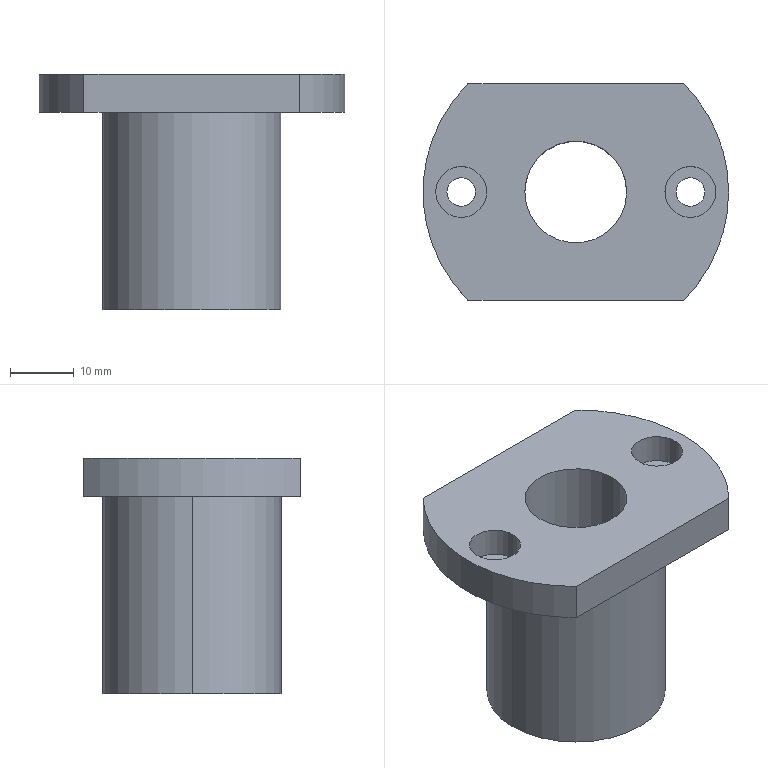Part | STEP file | LMH16UU | 1 solid | 22 faces | box 48 x 34 x 37 mm | volume 20039 mm3 | cylinder 15 | plane 7 | commonest cylinder face diameters 4.5 x4 8 x4 48 x3 16 x2 28 x2